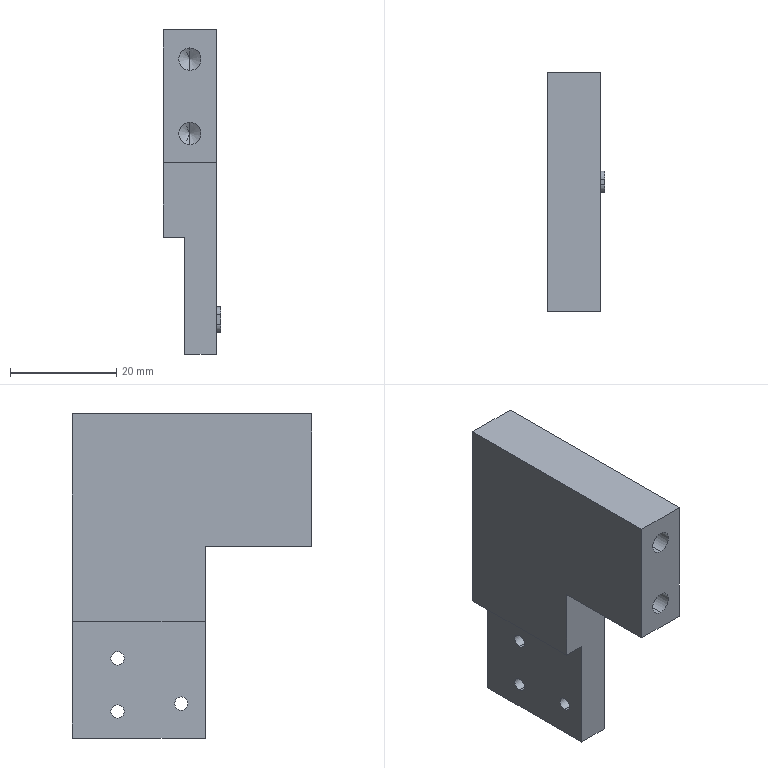Part | SolidWorks | features ICE 4, HoleWzd 3, ExtruThin 1, Fillet 1 | 1 solid | 33 faces | box 10.8 x 45 x 61 mm | volume 17616 mm3 | plane 15 | cylinder 14 | cone 4 | commonest cylinder face diameters 2.5 x6 3 x4 4.2 x4
STEP:
#1=CARTESIAN_POINT('',(10.8,24.5,-30.75));
#2=VERTEX_POINT('',#1);
#3=CARTESIAN_POINT('',(10.8,24.5,-28.25));
#4=VERTEX_POINT('',#3);
#5=CARTESIAN_POINT('',(10.8,24.5,-29.5));
#6=DIRECTION('',(-1.,0.,0.));
#7=DIRECTION('',(0.,0.,1.));
#8=AXIS2_PLACEMENT_3D('',#5,#6,#7);
#9=CIRCLE('',#8,1.25);
#10=EDGE_CURVE('',#2,#4,#9,.T.);
#11=ORIENTED_EDGE('',*,*,#10,.F.);
#12=CARTESIAN_POINT('',(4.,24.5,-30.75));
#13=VERTEX_POINT('',#12);
#14=CARTESIAN_POINT('',(0.,24.5,-30.75));
#15=DIRECTION('',(-1.,0.,0.));
#16=VECTOR('',#15,1000.);
#17=LINE('',#14,#16);
#18=EDGE_CURVE('',#2,#13,#17,.T.);
#19=ORIENTED_EDGE('',*,*,#18,.T.);
#20=CARTESIAN_POINT('',(4.,24.5,-28.25));
#21=VERTEX_POINT('',#20);
#22=CARTESIAN_POINT('',(4.,24.5,-29.5));
#23=DIRECTION('',(1.,0.,0.));
#24=DIRECTION('',(0.,0.,-1.));
#25=AXIS2_PLACEMENT_3D('',#22,#23,#24);
#26=CIRCLE('',#25,1.25);
#27=EDGE_CURVE('',#21,#13,#26,.T.);
#28=ORIENTED_EDGE('',*,*,#27,.F.);
#29=CARTESIAN_POINT('',(0.,24.5,-28.25));
#30=DIRECTION('',(-1.,0.,0.));
#31=VECTOR('',#30,1000.);
#32=LINE('',#29,#31);
#33=EDGE_CURVE('',#4,#21,#32,.T.);
#34=ORIENTED_EDGE('',*,*,#33,.F.);
#35=EDGE_LOOP('',(#11,#19,#28,#34));
#36=FACE_OUTER_BOUND('',#35,.T.);
#37=CARTESIAN_POINT('',(0.,24.5,-29.5));
#38=DIRECTION('',(-1.,0.,0.));
#39=DIRECTION('',(0.,0.,1.));
#40=AXIS2_PLACEMENT_3D('',#37,#38,#39);
#41=CYLINDRICAL_SURFACE('',#40,1.25);
#42=ADVANCED_FACE('',(#36),#41,.F.);
#43=CARTESIAN_POINT('',(4.,36.5,-19.75));
#44=VERTEX_POINT('',#43);
#45=CARTESIAN_POINT('',(4.,36.5,-22.25));
#46=VERTEX_POINT('',#45);
#47=CARTESIAN_POINT('',(4.,36.5,-21.));
#48=DIRECTION('',(1.,0.,0.));
#49=DIRECTION('',(0.,0.,-1.));
#50=AXIS2_PLACEMENT_3D('',#47,#48,#49);
#51=CIRCLE('',#50,1.25);
#52=EDGE_CURVE('',#44,#46,#51,.T.);
#53=ORIENTED_EDGE('',*,*,#52,.F.);
#54=CARTESIAN_POINT('',(10.,36.5,-19.75));
#55=VERTEX_POINT('',#54);
#56=CARTESIAN_POINT('',(10.,36.5,-19.75));
#57=DIRECTION('',(1.,0.,0.));
#58=VECTOR('',#57,1000.);
#59=LINE('',#56,#58);
#60=EDGE_CURVE('',#44,#55,#59,.T.);
#61=ORIENTED_EDGE('',*,*,#60,.T.);
#62=CARTESIAN_POINT('',(10.,36.5,-22.25));
#63=VERTEX_POINT('',#62);
#64=CARTESIAN_POINT('',(10.,36.5,-21.));
#65=DIRECTION('',(1.,0.,0.));
#66=DIRECTION('',(0.,0.,-1.));
#67=AXIS2_PLACEMENT_3D('',#64,#65,#66);
#68=CIRCLE('',#67,1.25);
#69=EDGE_CURVE('',#55,#63,#68,.T.);
#70=ORIENTED_EDGE('',*,*,#69,.T.);
#71=CARTESIAN_POINT('',(10.,36.5,-22.25));
#72=DIRECTION('',(1.,0.,0.));
#73=VECTOR('',#72,1000.);
#74=LINE('',#71,#73);
#75=EDGE_CURVE('',#46,#63,#74,.T.);
#76=ORIENTED_EDGE('',*,*,#75,.F.);
#77=EDGE_LOOP('',(#53,#61,#70,#76));
#78=FACE_OUTER_BOUND('',#77,.T.);
#79=CARTESIAN_POINT('',(10.,36.5,-21.));
#80=DIRECTION('',(1.,0.,0.));
#81=DIRECTION('',(0.,0.,-1.));
#82=AXIS2_PLACEMENT_3D('',#79,#80,#81);
#83=CYLINDRICAL_SURFACE('',#82,1.25);
#84=ADVANCED_FACE('',(#78),#83,.F.);
#85=CARTESIAN_POINT('',(4.,36.5,-29.75));
#86=VERTEX_POINT('',#85);
#87=CARTESIAN_POINT('',(4.,36.5,-32.25));
#88=VERTEX_POINT('',#87);
#89=CARTESIAN_POINT('',(4.,36.5,-31.));
#90=DIRECTION('',(1.,0.,0.));
#91=DIRECTION('',(0.,0.,-1.));
#92=AXIS2_PLACEMENT_3D('',#89,#90,#91);
#93=CIRCLE('',#92,1.25);
#94=EDGE_CURVE('',#86,#88,#93,.T.);
#95=ORIENTED_EDGE('',*,*,#94,.F.);
#96=CARTESIAN_POINT('',(10.,36.5,-29.75));
#97=VERTEX_POINT('',#96);
#98=CARTESIAN_POINT('',(10.,36.5,-29.75));
#99=DIRECTION('',(1.,0.,0.));
#100=VECTOR('',#99,1000.);
#101=LINE('',#98,#100);
#102=EDGE_CURVE('',#86,#97,#101,.T.);
#103=ORIENTED_EDGE('',*,*,#102,.T.);
#104=CARTESIAN_POINT('',(10.,36.5,-32.25));
#105=VERTEX_POINT('',#104);
#106=CARTESIAN_POINT('',(10.,36.5,-31.));
#107=DIRECTION('',(1.,0.,0.));
#108=DIRECTION('',(0.,0.,-1.));
#109=AXIS2_PLACEMENT_3D('',#106,#107,#108);
#110=CIRCLE('',#109,1.25);
#111=EDGE_CURVE('',#97,#105,#110,.T.);
#112=ORIENTED_EDGE('',*,*,#111,.T.);
#113=CARTESIAN_POINT('',(10.,36.5,-32.25));
#114=DIRECTION('',(1.,0.,0.));
#115=VECTOR('',#114,1000.);
#116=LINE('',#113,#115);
#117=EDGE_CURVE('',#88,#105,#116,.T.);
#118=ORIENTED_EDGE('',*,*,#117,.F.);
#119=EDGE_LOOP('',(#95,#103,#112,#118));
#120=FACE_OUTER_BOUND('',#119,.T.);
#121=CARTESIAN_POINT('',(10.,36.5,-31.));
#122=DIRECTION('',(1.,0.,0.));
#123=DIRECTION('',(0.,0.,-1.));
#124=AXIS2_PLACEMENT_3D('',#121,#122,#123);
#125=CYLINDRICAL_SURFACE('',#124,1.25);
#126=ADVANCED_FACE('',(#120),#125,.F.);
#127=CARTESIAN_POINT('',(5.,12.4,7.6));
#128=VERTEX_POINT('',#127);
#129=CARTESIAN_POINT('',(5.,12.4,3.4));
#130=VERTEX_POINT('',#129);
#131=CARTESIAN_POINT('',(5.,12.4,5.5));
#132=DIRECTION('',(0.,-1.,0.));
#133=DIRECTION('',(0.,0.,-1.));
#134=AXIS2_PLACEMENT_3D('',#131,#132,#133);
#135=CIRCLE('',#134,2.1);
#136=EDGE_CURVE('',#128,#130,#135,.T.);
#137=ORIENTED_EDGE('',*,*,#136,.F.);
#138=CARTESIAN_POINT('',(5.,0.,7.6));
#139=VERTEX_POINT('',#138);
#140=CARTESIAN_POINT('',(5.,0.,7.6));
#141=DIRECTION('',(0.,-1.,0.));
#142=VECTOR('',#141,1000.);
#143=LINE('',#140,#142);
#144=EDGE_CURVE('',#128,#139,#143,.T.);
#145=ORIENTED_EDGE('',*,*,#144,.T.);
#146=CARTESIAN_POINT('',(5.,0.,3.4));
#147=VERTEX_POINT('',#146);
#148=CARTESIAN_POINT('',(5.,0.,5.5));
#149=DIRECTION('',(0.,-1.,0.));
#150=DIRECTION('',(0.,0.,-1.));
#151=AXIS2_PLACEMENT_3D('',#148,#149,#150);
#152=CIRCLE('',#151,2.1);
#153=EDGE_CURVE('',#139,#147,#152,.T.);
#154=ORIENTED_EDGE('',*,*,#153,.T.);
#155=CARTESIAN_POINT('',(5.,0.,3.4));
#156=DIRECTION('',(0.,-1.,0.));
#157=VECTOR('',#156,1000.);
#158=LINE('',#155,#157);
#159=EDGE_CURVE('',#130,#147,#158,.T.);
#160=ORIENTED_EDGE('',*,*,#159,.F.);
#161=EDGE_LOOP('',(#137,#145,#154,#160));
#162=FACE_OUTER_BOUND('',#161,.T.);
#163=CARTESIAN_POINT('',(5.,0.,5.5));
#164=DIRECTION('',(0.,-1.,0.));
#165=DIRECTION('',(0.,0.,-1.));
#166=AXIS2_PLACEMENT_3D('',#163,#164,#165);
#167=CYLINDRICAL_SURFACE('',#166,2.1);
#168=ADVANCED_FACE('',(#162),#167,.F.);
#169=CARTESIAN_POINT('',(5.,13.662,5.5));
#170=VERTEX_POINT('',#169);
#171=CARTESIAN_POINT('',(5.,12.4,3.4));
#172=DIRECTION('',(0.,-0.515,-0.8572));
#173=VECTOR('',#172,1000.);
#174=LINE('',#171,#173);
#175=EDGE_CURVE('',#170,#130,#174,.T.);
#176=ORIENTED_EDGE('',*,*,#175,.F.);
#177=CARTESIAN_POINT('',(5.,12.4,7.6));
#178=DIRECTION('',(0.,-0.515,0.8572));
#179=VECTOR('',#178,1000.);
#180=LINE('',#177,#179);
#181=EDGE_CURVE('',#170,#128,#180,.T.);
#182=ORIENTED_EDGE('',*,*,#181,.T.);
#183=ORIENTED_EDGE('',*,*,#136,.T.);
#184=EDGE_LOOP('',(#176,#182,#183));
#185=FACE_OUTER_BOUND('',#184,.T.);
#186=CARTESIAN_POINT('',(5.,12.4,5.5));
#187=DIRECTION('',(0.,-1.,0.));
#188=DIRECTION('',(0.,0.,-1.));
#189=AXIS2_PLACEMENT_3D('',#186,#187,#188);
#190=CONICAL_SURFACE('',#189,2.1,1.03);
#191=ADVANCED_FACE('',(#185),#190,.F.);
#192=CARTESIAN_POINT('',(5.,12.4,21.6));
#193=VERTEX_POINT('',#192);
#194=CARTESIAN_POINT('',(5.,12.4,17.4));
#195=VERTEX_POINT('',#194);
#196=CARTESIAN_POINT('',(5.,12.4,19.5));
#197=DIRECTION('',(0.,-1.,0.));
#198=DIRECTION('',(0.,0.,-1.));
#199=AXIS2_PLACEMENT_3D('',#196,#197,#198);
#200=CIRCLE('',#199,2.1);
#201=EDGE_CURVE('',#193,#195,#200,.T.);
#202=ORIENTED_EDGE('',*,*,#201,.F.);
#203=CARTESIAN_POINT('',(5.,0.,21.6));
#204=VERTEX_POINT('',#203);
#205=CARTESIAN_POINT('',(5.,0.,21.6));
#206=DIRECTION('',(0.,-1.,0.));
#207=VECTOR('',#206,1000.);
#208=LINE('',#205,#207);
#209=EDGE_CURVE('',#193,#204,#208,.T.);
#210=ORIENTED_EDGE('',*,*,#209,.T.);
#211=CARTESIAN_POINT('',(5.,0.,17.4));
#212=VERTEX_POINT('',#211);
#213=CARTESIAN_POINT('',(5.,0.,19.5));
#214=DIRECTION('',(0.,-1.,0.));
#215=DIRECTION('',(0.,0.,-1.));
#216=AXIS2_PLACEMENT_3D('',#213,#214,#215);
#217=CIRCLE('',#216,2.1);
#218=EDGE_CURVE('',#204,#212,#217,.T.);
#219=ORIENTED_EDGE('',*,*,#218,.T.);
#220=CARTESIAN_POINT('',(5.,0.,17.4));
#221=DIRECTION('',(0.,-1.,0.));
#222=VECTOR('',#221,1000.);
#223=LINE('',#220,#222);
#224=EDGE_CURVE('',#195,#212,#223,.T.);
#225=ORIENTED_EDGE('',*,*,#224,.F.);
#226=EDGE_LOOP('',(#202,#210,#219,#225));
#227=FACE_OUTER_BOUND('',#226,.T.);
#228=CARTESIAN_POINT('',(5.,0.,19.5));
#229=DIRECTION('',(0.,-1.,0.));
#230=DIRECTION('',(0.,0.,-1.));
#231=AXIS2_PLACEMENT_3D('',#228,#229,#230);
#232=CYLINDRICAL_SURFACE('',#231,2.1);
#233=ADVANCED_FACE('',(#227),#232,.F.);
#234=CARTESIAN_POINT('',(5.,13.662,19.5));
#235=VERTEX_POINT('',#234);
#236=CARTESIAN_POINT('',(5.,12.4,17.4));
#237=DIRECTION('',(0.,-0.515,-0.8572));
#238=VECTOR('',#237,1000.);
#239=LINE('',#236,#238);
#240=EDGE_CURVE('',#235,#195,#239,.T.);
#241=ORIENTED_EDGE('',*,*,#240,.F.);
#242=CARTESIAN_POINT('',(5.,12.4,21.6));
#243=DIRECTION('',(0.,-0.515,0.8572));
#244=VECTOR('',#243,1000.);
#245=LINE('',#242,#244);
#246=EDGE_CURVE('',#235,#193,#245,.T.);
#247=ORIENTED_EDGE('',*,*,#246,.T.);
#248=ORIENTED_EDGE('',*,*,#201,.T.);
#249=EDGE_LOOP('',(#241,#247,#248));
#250=FACE_OUTER_BOUND('',#249,.T.);
#251=CARTESIAN_POINT('',(5.,12.4,19.5));
#252=DIRECTION('',(0.,-1.,0.));
#253=DIRECTION('',(0.,0.,-1.));
#254=AXIS2_PLACEMENT_3D('',#251,#252,#253);
#255=CONICAL_SURFACE('',#254,2.1,1.03);
#256=ADVANCED_FACE('',(#250),#255,.F.);
#257=CARTESIAN_POINT('',(10.,0.,0.));
#258=VERTEX_POINT('',#257);
#259=CARTESIAN_POINT('',(10.,0.,25.));
#260=VERTEX_POINT('',#259);
#261=CARTESIAN_POINT('',(10.,0.,25.));
#262=DIRECTION('',(0.,0.,1.));
#263=VECTOR('',#262,1000.);
#264=LINE('',#261,#263);
#265=EDGE_CURVE('',#258,#260,#264,.T.);
#266=ORIENTED_EDGE('',*,*,#265,.F.);
#267=CARTESIAN_POINT('',(10.,20.,0.));
#268=VERTEX_POINT('',#267);
#269=CARTESIAN_POINT('',(10.,0.,0.));
#270=DIRECTION('',(0.,1.,0.));
#271=VECTOR('',#270,1000.);
#272=LINE('',#269,#271);
#273=EDGE_CURVE('',#258,#268,#272,.T.);
#274=ORIENTED_EDGE('',*,*,#273,.T.);
#275=CARTESIAN_POINT('',(10.,20.,-36.));
#276=VERTEX_POINT('',#275);
#277=CARTESIAN_POINT('',(10.,20.,0.));
#278=DIRECTION('',(0.,0.,-1.));
#279=VECTOR('',#278,1000.);
#280=LINE('',#277,#279);
#281=EDGE_CURVE('',#268,#276,#280,.T.);
#282=ORIENTED_EDGE('',*,*,#281,.T.);
#283=CARTESIAN_POINT('',(10.,45.,-36.));
#284=VERTEX_POINT('',#283);
#285=CARTESIAN_POINT('',(10.,45.,-36.));
#286=DIRECTION('',(0.,1.,0.));
#287=VECTOR('',#286,1000.);
#288=LINE('',#285,#287);
#289=EDGE_CURVE('',#276,#284,#288,.T.);
#290=ORIENTED_EDGE('',*,*,#289,.T.);
#291=CARTESIAN_POINT('',(10.,45.,25.));
#292=VERTEX_POINT('',#291);
#293=CARTESIAN_POINT('',(10.,45.,25.));
#294=DIRECTION('',(0.,0.,-1.));
#295=VECTOR('',#294,1000.);
#296=LINE('',#293,#295);
#297=EDGE_CURVE('',#292,#284,#296,.T.);
#298=ORIENTED_EDGE('',*,*,#297,.F.);
#299=CARTESIAN_POINT('',(10.,0.,25.));
#300=DIRECTION('',(0.,1.,0.));
#301=VECTOR('',#300,1000.);
#302=LINE('',#299,#301);
#303=EDGE_CURVE('',#260,#292,#302,.T.);
#304=ORIENTED_EDGE('',*,*,#303,.F.);
#305=EDGE_LOOP('',(#266,#274,#282,#290,#298,#304));
#306=FACE_OUTER_BOUND('',#305,.T.);
#307=CARTESIAN_POINT('',(10.,36.5,-31.));
#308=DIRECTION('',(1.,0.,0.));
#309=DIRECTION('',(0.,0.,-1.));
#310=AXIS2_PLACEMENT_3D('',#307,#308,#309);
#311=CIRCLE('',#310,1.25);
#312=EDGE_CURVE('',#105,#97,#311,.T.);
#313=ORIENTED_EDGE('',*,*,#312,.F.);
#314=ORIENTED_EDGE('',*,*,#111,.F.);
#315=EDGE_LOOP('',(#313,#314));
#316=FACE_BOUND('',#315,.T.);
#317=CARTESIAN_POINT('',(10.,36.5,-21.));
#318=DIRECTION('',(1.,0.,0.));
#319=DIRECTION('',(0.,0.,-1.));
#320=AXIS2_PLACEMENT_3D('',#317,#318,#319);
#321=CIRCLE('',#320,1.25);
#322=EDGE_CURVE('',#63,#55,#321,.T.);
#323=ORIENTED_EDGE('',*,*,#322,.F.);
#324=ORIENTED_EDGE('',*,*,#69,.F.);
#325=EDGE_LOOP('',(#323,#324));
#326=FACE_BOUND('',#325,.T.);
#327=CARTESIAN_POINT('',(10.,24.,-31.9));
#328=VERTEX_POINT('',#327);
#329=CARTESIAN_POINT('',(10.,25.,-31.9));
#330=VERTEX_POINT('',#329);
#331=CARTESIAN_POINT('',(10.,26.5,-31.9));
#332=DIRECTION('',(0.,1.,0.));
#333=VECTOR('',#332,1000.);
#334=LINE('',#331,#333);
#335=EDGE_CURVE('',#328,#330,#334,.T.);
#336=ORIENTED_EDGE('',*,*,#335,.F.);
#337=CARTESIAN_POINT('',(10.,22.5,-30.4));
#338=VERTEX_POINT('',#337);
#339=CARTESIAN_POINT('',(10.,24.,-30.4));
#340=DIRECTION('',(-1.,0.,0.));
#341=DIRECTION('',(0.,0.,1.));
#342=AXIS2_PLACEMENT_3D('',#339,#340,#341);
#343=CIRCLE('',#342,1.5);
#344=EDGE_CURVE('',#328,#338,#343,.T.);
#345=ORIENTED_EDGE('',*,*,#344,.T.);
#346=CARTESIAN_POINT('',(10.,22.5,-28.6));
#347=VERTEX_POINT('',#346);
#348=CARTESIAN_POINT('',(10.,22.5,-27.1));
#349=DIRECTION('',(0.,0.,-1.));
#350=VECTOR('',#349,1000.);
#351=LINE('',#348,#350);
#352=EDGE_CURVE('',#347,#338,#351,.T.);
#353=ORIENTED_EDGE('',*,*,#352,.F.);
#354=CARTESIAN_POINT('',(10.,24.,-27.1));
#355=VERTEX_POINT('',#354);
#356=CARTESIAN_POINT('',(10.,24.,-28.6));
#357=DIRECTION('',(-1.,0.,0.));
#358=DIRECTION('',(0.,0.,1.));
#359=AXIS2_PLACEMENT_3D('',#356,#357,#358);
#360=CIRCLE('',#359,1.5);
#361=EDGE_CURVE('',#347,#355,#360,.T.);
#362=ORIENTED_EDGE('',*,*,#361,.T.);
#363=CARTESIAN_POINT('',(10.,25.,-27.1));
#364=VERTEX_POINT('',#363);
#365=CARTESIAN_POINT('',(10.,26.5,-27.1));
#366=DIRECTION('',(0.,-1.,0.));
#367=VECTOR('',#366,1000.);
#368=LINE('',#365,#367);
#369=EDGE_CURVE('',#364,#355,#368,.T.);
#370=ORIENTED_EDGE('',*,*,#369,.F.);
#371=CARTESIAN_POINT('',(10.,26.5,-28.6));
#372=VERTEX_POINT('',#371);
#373=CARTESIAN_POINT('',(10.,25.,-28.6));
#374=DIRECTION('',(-1.,0.,0.));
#375=DIRECTION('',(0.,0.,1.));
#376=AXIS2_PLACEMENT_3D('',#373,#374,#375);
#377=CIRCLE('',#376,1.5);
#378=EDGE_CURVE('',#364,#372,#377,.T.);
#379=ORIENTED_EDGE('',*,*,#378,.T.);
#380=CARTESIAN_POINT('',(10.,26.5,-30.4));
#381=VERTEX_POINT('',#380);
#382=CARTESIAN_POINT('',(10.,26.5,-27.1));
#383=DIRECTION('',(0.,0.,1.));
#384=VECTOR('',#383,1000.);
#385=LINE('',#382,#384);
#386=EDGE_CURVE('',#381,#372,#385,.T.);
#387=ORIENTED_EDGE('',*,*,#386,.F.);
#388=CARTESIAN_POINT('',(10.,25.,-30.4));
#389=DIRECTION('',(-1.,0.,0.));
#390=DIRECTION('',(0.,0.,1.));
#391=AXIS2_PLACEMENT_3D('',#388,#389,#390);
#392=CIRCLE('',#391,1.5);
#393=EDGE_CURVE('',#381,#330,#392,.T.);
#394=ORIENTED_EDGE('',*,*,#393,.T.);
#395=EDGE_LOOP('',(#336,#345,#353,#362,#370,#379,#387,#394));
#396=FACE_BOUND('',#395,.T.);
#397=CARTESIAN_POINT('',(10.,0.,25.));
#398=DIRECTION('',(-1.,0.,0.));
#399=DIRECTION('',(0.,0.,1.));
#400=AXIS2_PLACEMENT_3D('',#397,#398,#399);
#401=PLANE('',#400);
#402=ADVANCED_FACE('',(#306,#316,#326,#396),#401,.F.);
#403=CARTESIAN_POINT('',(0.,0.,25.));
#404=VERTEX_POINT('',#403);
#405=CARTESIAN_POINT('',(0.,0.,25.));
#406=DIRECTION('',(-1.,0.,0.));
#407=VECTOR('',#406,1000.);
#408=LINE('',#405,#407);
#409=EDGE_CURVE('',#260,#404,#408,.T.);
#410=ORIENTED_EDGE('',*,*,#409,.F.);
#411=ORIENTED_EDGE('',*,*,#303,.T.);
#412=CARTESIAN_POINT('',(0.,45.,25.));
#413=VERTEX_POINT('',#412);
#414=CARTESIAN_POINT('',(0.,45.,25.));
#415=DIRECTION('',(1.,0.,0.));
#416=VECTOR('',#415,1000.);
#417=LINE('',#414,#416);
#418=EDGE_CURVE('',#413,#292,#417,.T.);
#419=ORIENTED_EDGE('',*,*,#418,.F.);
#420=CARTESIAN_POINT('',(0.,0.,25.));
#421=DIRECTION('',(0.,1.,0.));
#422=VECTOR('',#421,1000.);
#423=LINE('',#420,#422);
#424=EDGE_CURVE('',#404,#413,#423,.T.);
#425=ORIENTED_EDGE('',*,*,#424,.F.);
#426=EDGE_LOOP('',(#410,#411,#419,#425));
#427=FACE_OUTER_BOUND('',#426,.T.);
#428=CARTESIAN_POINT('',(0.,0.,25.));
#429=DIRECTION('',(0.,0.,-1.));
#430=DIRECTION('',(-1.,0.,0.));
#431=AXIS2_PLACEMENT_3D('',#428,#429,#430);
#432=PLANE('',#431);
#433=ADVANCED_FACE('',(#427),#432,.F.);
#434=ORIENTED_EDGE('',*,*,#273,.F.);
#435=CARTESIAN_POINT('',(0.,0.,0.));
#436=VERTEX_POINT('',#435);
#437=CARTESIAN_POINT('',(0.,0.,0.));
#438=DIRECTION('',(-1.,0.,0.));
#439=VECTOR('',#438,1000.);
#440=LINE('',#437,#439);
#441=EDGE_CURVE('',#258,#436,#440,.T.);
#442=ORIENTED_EDGE('',*,*,#441,.T.);
#443=CARTESIAN_POINT('',(0.,20.,0.));
#444=VERTEX_POINT('',#443);
#445=CARTESIAN_POINT('',(0.,0.,0.));
#446=DIRECTION('',(0.,1.,0.));
#447=VECTOR('',#446,1000.);
#448=LINE('',#445,#447);
#449=EDGE_CURVE('',#436,#444,#448,.T.);
#450=ORIENTED_EDGE('',*,*,#449,.T.);
#451=CARTESIAN_POINT('',(53.829,20.,0.));
#452=DIRECTION('',(-1.,0.,0.));
#453=VECTOR('',#452,1000.);
#454=LINE('',#451,#453);
#455=EDGE_CURVE('',#268,#444,#454,.T.);
#456=ORIENTED_EDGE('',*,*,#455,.F.);
#457=EDGE_LOOP('',(#434,#442,#450,#456));
#458=FACE_OUTER_BOUND('',#457,.T.);
#459=CARTESIAN_POINT('',(0.,0.,0.));
#460=DIRECTION('',(0.,0.,-1.));
#461=DIRECTION('',(-1.,0.,0.));
#462=AXIS2_PLACEMENT_3D('',#459,#460,#461);
#463=PLANE('',#462);
#464=ADVANCED_FACE('',(#458),#463,.T.);
#465=CARTESIAN_POINT('',(4.,45.,-14.));
#466=VERTEX_POINT('',#465);
#467=CARTESIAN_POINT('',(4.,45.,-36.));
#468=VERTEX_POINT('',#467);
#469=CARTESIAN_POINT('',(4.,45.,-36.));
#470=DIRECTION('',(0.,0.,-1.));
#471=VECTOR('',#470,1000.);
#472=LINE('',#469,#471);
#473=EDGE_CURVE('',#466,#468,#472,.T.);
#474=ORIENTED_EDGE('',*,*,#473,.F.);
#475=CARTESIAN_POINT('',(0.,45.,-14.));
#476=VERTEX_POINT('',#475);
#477=CARTESIAN_POINT('',(0.,45.,-14.));
#478=DIRECTION('',(1.,0.,0.));
#479=VECTOR('',#478,1000.);
#480=LINE('',#477,#479);
#481=EDGE_CURVE('',#476,#466,#480,.T.);
#482=ORIENTED_EDGE('',*,*,#481,.F.);
#483=CARTESIAN_POINT('',(0.,45.,25.));
#484=DIRECTION('',(0.,0.,-1.));
#485=VECTOR('',#484,1000.);
#486=LINE('',#483,#485);
#487=EDGE_CURVE('',#413,#476,#486,.T.);
#488=ORIENTED_EDGE('',*,*,#487,.F.);
#489=ORIENTED_EDGE('',*,*,#418,.T.);
#490=ORIENTED_EDGE('',*,*,#297,.T.);
#491=CARTESIAN_POINT('',(53.829,45.,-36.));
#492=DIRECTION('',(-1.,0.,0.));
#493=VECTOR('',#492,1000.);
#494=LINE('',#491,#493);
#495=EDGE_CURVE('',#284,#468,#494,.T.);
#496=ORIENTED_EDGE('',*,*,#495,.T.);
#497=EDGE_LOOP('',(#474,#482,#488,#489,#490,#496));
#498=FACE_OUTER_BOUND('',#497,.T.);
#499=CARTESIAN_POINT('',(0.,45.,25.));
#500=DIRECTION('',(0.,1.,0.));
#501=DIRECTION('',(0.,0.,1.));
#502=AXIS2_PLACEMENT_3D('',#499,#500,#501);
#503=PLANE('',#502);
#504=ADVANCED_FACE('',(#498),#503,.T.);
#505=CARTESIAN_POINT('',(0.,20.,-14.));
#506=VERTEX_POINT('',#505);
#507=CARTESIAN_POINT('',(0.,-10.,-14.));
#508=DIRECTION('',(0.,1.,0.));
#509=VECTOR('',#508,1000.);
#510=LINE('',#507,#509);
#511=EDGE_CURVE('',#506,#476,#510,.T.);
#512=ORIENTED_EDGE('',*,*,#511,.F.);
#513=CARTESIAN_POINT('',(0.,20.,0.));
#514=DIRECTION('',(0.,0.,1.));
#515=VECTOR('',#514,1000.);
#516=LINE('',#513,#515);
#517=EDGE_CURVE('',#506,#444,#516,.T.);
#518=ORIENTED_EDGE('',*,*,#517,.T.);
#519=ORIENTED_EDGE('',*,*,#449,.F.);
#520=CARTESIAN_POINT('',(0.,0.,25.));
#521=DIRECTION('',(0.,0.,-1.));
#522=VECTOR('',#521,1000.);
#523=LINE('',#520,#522);
#524=EDGE_CURVE('',#404,#436,#523,.T.);
#525=ORIENTED_EDGE('',*,*,#524,.F.);
#526=ORIENTED_EDGE('',*,*,#424,.T.);
#527=ORIENTED_EDGE('',*,*,#487,.T.);
#528=EDGE_LOOP('',(#512,#518,#519,#525,#526,#527));
#529=FACE_OUTER_BOUND('',#528,.T.);
#530=CARTESIAN_POINT('',(0.,0.,25.));
#531=DIRECTION('',(-1.,0.,0.));
#532=DIRECTION('',(0.,0.,1.));
#533=AXIS2_PLACEMENT_3D('',#530,#531,#532);
#534=PLANE('',#533);
#535=ADVANCED_FACE('',(#529),#534,.T.);
#536=CARTESIAN_POINT('',(4.,20.,-36.));
#537=VERTEX_POINT('',#536);
#538=CARTESIAN_POINT('',(4.,20.,-14.));
#539=VERTEX_POINT('',#538);
#540=CARTESIAN_POINT('',(4.,20.,0.));
#541=DIRECTION('',(0.,0.,1.));
#542=VECTOR('',#541,1000.);
#543=LINE('',#540,#542);
#544=EDGE_CURVE('',#537,#539,#543,.T.);
#545=ORIENTED_EDGE('',*,*,#544,.F.);
#546=CARTESIAN_POINT('',(53.829,20.,-36.));
#547=DIRECTION('',(-1.,0.,0.));
#548=VECTOR('',#547,1000.);
#549=LINE('',#546,#548);
#550=EDGE_CURVE('',#276,#537,#549,.T.);
#551=ORIENTED_EDGE('',*,*,#550,.F.);
#552=ORIENTED_EDGE('',*,*,#281,.F.);
#553=ORIENTED_EDGE('',*,*,#455,.T.);
#554=ORIENTED_EDGE('',*,*,#517,.F.);
#555=CARTESIAN_POINT('',(53.829,20.,-14.));
#556=DIRECTION('',(-1.,0.,0.));
#557=VECTOR('',#556,1000.);
#558=LINE('',#555,#557);
#559=EDGE_CURVE('',#539,#506,#558,.T.);
#560=ORIENTED_EDGE('',*,*,#559,.F.);
#561=EDGE_LOOP('',(#545,#551,#552,#553,#554,#560));
#562=FACE_OUTER_BOUND('',#561,.T.);
#563=CARTESIAN_POINT('',(53.829,20.,0.));
#564=DIRECTION('',(0.,-1.,0.));
#565=DIRECTION('',(0.,0.,-1.));
#566=AXIS2_PLACEMENT_3D('',#563,#564,#565);
#567=PLANE('',#566);
#568=ADVANCED_FACE('',(#562),#567,.T.);
#569=CARTESIAN_POINT('',(4.,45.,-36.));
#570=DIRECTION('',(0.,-1.,0.));
#571=VECTOR('',#570,1000.);
#572=LINE('',#569,#571);
#573=EDGE_CURVE('',#468,#537,#572,.T.);
#574=ORIENTED_EDGE('',*,*,#573,.F.);
#575=ORIENTED_EDGE('',*,*,#495,.F.);
#576=ORIENTED_EDGE('',*,*,#289,.F.);
#577=ORIENTED_EDGE('',*,*,#550,.T.);
#578=EDGE_LOOP('',(#574,#575,#576,#577));
#579=FACE_OUTER_BOUND('',#578,.T.);
#580=CARTESIAN_POINT('',(53.829,45.,-36.));
#581=DIRECTION('',(0.,0.,-1.));
#582=DIRECTION('',(0.,1.,0.));
#583=AXIS2_PLACEMENT_3D('',#580,#581,#582);
#584=PLANE('',#583);
#585=ADVANCED_FACE('',(#579),#584,.T.);
#586=ORIENTED_EDGE('',*,*,#27,.T.);
#587=CARTESIAN_POINT('',(4.,24.5,-29.5));
#588=DIRECTION('',(1.,0.,0.));
#589=DIRECTION('',(0.,0.,-1.));
#590=AXIS2_PLACEMENT_3D('',#587,#588,#589);
#591=CIRCLE('',#590,1.25);
#592=EDGE_CURVE('',#13,#21,#591,.T.);
#593=ORIENTED_EDGE('',*,*,#592,.T.);
#594=EDGE_LOOP('',(#586,#593));
#595=FACE_BOUND('',#594,.T.);
#596=CARTESIAN_POINT('',(4.,36.5,-21.));
#597=DIRECTION('',(1.,0.,0.));
#598=DIRECTION('',(0.,0.,-1.));
#599=AXIS2_PLACEMENT_3D('',#596,#597,#598);
#600=CIRCLE('',#599,1.25);
#601=EDGE_CURVE('',#46,#44,#600,.T.);
#602=ORIENTED_EDGE('',*,*,#601,.T.);
#603=ORIENTED_EDGE('',*,*,#52,.T.);
#604=EDGE_LOOP('',(#602,#603));
#605=FACE_BOUND('',#604,.T.);
#606=CARTESIAN_POINT('',(4.,36.5,-31.));
#607=DIRECTION('',(1.,0.,0.));
#608=DIRECTION('',(0.,0.,-1.));
#609=AXIS2_PLACEMENT_3D('',#606,#607,#608);
#610=CIRCLE('',#609,1.25);
#611=EDGE_CURVE('',#88,#86,#610,.T.);
#612=ORIENTED_EDGE('',*,*,#611,.T.);
#613=ORIENTED_EDGE('',*,*,#94,.T.);
#614=EDGE_LOOP('',(#612,#613));
#615=FACE_BOUND('',#614,.T.);
#616=ORIENTED_EDGE('',*,*,#544,.T.);
#617=CARTESIAN_POINT('',(4.,-10.,-14.));
#618=DIRECTION('',(0.,1.,0.));
#619=VECTOR('',#618,1000.);
#620=LINE('',#617,#619);
#621=EDGE_CURVE('',#539,#466,#620,.T.);
#622=ORIENTED_EDGE('',*,*,#621,.T.);
#623=ORIENTED_EDGE('',*,*,#473,.T.);
#624=ORIENTED_EDGE('',*,*,#573,.T.);
#625=EDGE_LOOP('',(#616,#622,#623,#624));
#626=FACE_OUTER_BOUND('',#625,.T.);
#627=CARTESIAN_POINT('',(4.,-10.,-36.));
#628=DIRECTION('',(1.,0.,0.));
#629=DIRECTION('',(0.,0.,-1.));
#630=AXIS2_PLACEMENT_3D('',#627,#628,#629);
#631=PLANE('',#630);
#632=ADVANCED_FACE('',(#595,#605,#615,#626),#631,.F.);
#633=ORIENTED_EDGE('',*,*,#559,.T.);
#634=ORIENTED_EDGE('',*,*,#511,.T.);
#635=ORIENTED_EDGE('',*,*,#481,.T.);
#636=ORIENTED_EDGE('',*,*,#621,.F.);
#637=EDGE_LOOP('',(#633,#634,#635,#636));
#638=FACE_OUTER_BOUND('',#637,.T.);
#639=CARTESIAN_POINT('',(0.,-10.,-14.));
#640=DIRECTION('',(0.,0.,1.));
#641=DIRECTION('',(1.,0.,0.));
#642=AXIS2_PLACEMENT_3D('',#639,#640,#641);
#643=PLANE('',#642);
#644=ADVANCED_FACE('',(#638),#643,.F.);
#645=CARTESIAN_POINT('',(5.,0.,5.5));
#646=DIRECTION('',(0.,-1.,0.));
#647=DIRECTION('',(0.,0.,-1.));
#648=AXIS2_PLACEMENT_3D('',#645,#646,#647);
#649=CIRCLE('',#648,2.1);
#650=EDGE_CURVE('',#147,#139,#649,.T.);
#651=ORIENTED_EDGE('',*,*,#650,.F.);
#652=ORIENTED_EDGE('',*,*,#153,.F.);
#653=EDGE_LOOP('',(#651,#652));
#654=FACE_BOUND('',#653,.T.);
#655=CARTESIAN_POINT('',(5.,0.,19.5));
#656=DIRECTION('',(0.,-1.,0.));
#657=DIRECTION('',(0.,0.,-1.));
#658=AXIS2_PLACEMENT_3D('',#655,#656,#657);
#659=CIRCLE('',#658,2.1);
#660=EDGE_CURVE('',#212,#204,#659,.T.);
#661=ORIENTED_EDGE('',*,*,#660,.F.);
#662=ORIENTED_EDGE('',*,*,#218,.F.);
#663=EDGE_LOOP('',(#661,#662));
#664=FACE_BOUND('',#663,.T.);
#665=ORIENTED_EDGE('',*,*,#441,.F.);
#666=ORIENTED_EDGE('',*,*,#265,.T.);
#667=ORIENTED_EDGE('',*,*,#409,.T.);
#668=ORIENTED_EDGE('',*,*,#524,.T.);
#669=EDGE_LOOP('',(#665,#666,#667,#668));
#670=FACE_OUTER_BOUND('',#669,.T.);
#671=CARTESIAN_POINT('',(0.,0.,0.));
#672=DIRECTION('',(0.,-1.,0.));
#673=DIRECTION('',(0.,0.,-1.));
#674=AXIS2_PLACEMENT_3D('',#671,#672,#673);
#675=PLANE('',#674);
#676=ADVANCED_FACE('',(#654,#664,#670),#675,.T.);
#677=ORIENTED_EDGE('',*,*,#246,.F.);
#678=ORIENTED_EDGE('',*,*,#240,.T.);
#679=CARTESIAN_POINT('',(5.,12.4,19.5));
#680=DIRECTION('',(0.,-1.,0.));
#681=DIRECTION('',(0.,0.,-1.));
#682=AXIS2_PLACEMENT_3D('',#679,#680,#681);
#683=CIRCLE('',#682,2.1);
#684=EDGE_CURVE('',#195,#193,#683,.T.);
#685=ORIENTED_EDGE('',*,*,#684,.T.);
#686=EDGE_LOOP('',(#677,#678,#685));
#687=FACE_OUTER_BOUND('',#686,.T.);
#688=CARTESIAN_POINT('',(5.,12.4,19.5));
#689=DIRECTION('',(0.,-1.,0.));
#690=DIRECTION('',(0.,0.,-1.));
#691=AXIS2_PLACEMENT_3D('',#688,#689,#690);
#692=CONICAL_SURFACE('',#691,2.1,1.03);
#693=ADVANCED_FACE('',(#687),#692,.F.);
#694=ORIENTED_EDGE('',*,*,#209,.F.);
#695=ORIENTED_EDGE('',*,*,#684,.F.);
#696=ORIENTED_EDGE('',*,*,#224,.T.);
#697=ORIENTED_EDGE('',*,*,#660,.T.);
#698=EDGE_LOOP('',(#694,#695,#696,#697));
#699=FACE_OUTER_BOUND('',#698,.T.);
#700=CARTESIAN_POINT('',(5.,0.,19.5));
#701=DIRECTION('',(0.,-1.,0.));
#702=DIRECTION('',(0.,0.,-1.));
#703=AXIS2_PLACEMENT_3D('',#700,#701,#702);
#704=CYLINDRICAL_SURFACE('',#703,2.1);
#705=ADVANCED_FACE('',(#699),#704,.F.);
#706=ORIENTED_EDGE('',*,*,#181,.F.);
#707=ORIENTED_EDGE('',*,*,#175,.T.);
#708=CARTESIAN_POINT('',(5.,12.4,5.5));
#709=DIRECTION('',(0.,-1.,0.));
#710=DIRECTION('',(0.,0.,-1.));
#711=AXIS2_PLACEMENT_3D('',#708,#709,#710);
#712=CIRCLE('',#711,2.1);
#713=EDGE_CURVE('',#130,#128,#712,.T.);
#714=ORIENTED_EDGE('',*,*,#713,.T.);
#715=EDGE_LOOP('',(#706,#707,#714));
#716=FACE_OUTER_BOUND('',#715,.T.);
#717=CARTESIAN_POINT('',(5.,12.4,5.5));
#718=DIRECTION('',(0.,-1.,0.));
#719=DIRECTION('',(0.,0.,-1.));
#720=AXIS2_PLACEMENT_3D('',#717,#718,#719);
#721=CONICAL_SURFACE('',#720,2.1,1.03);
#722=ADVANCED_FACE('',(#716),#721,.F.);
#723=ORIENTED_EDGE('',*,*,#144,.F.);
#724=ORIENTED_EDGE('',*,*,#713,.F.);
#725=ORIENTED_EDGE('',*,*,#159,.T.);
#726=ORIENTED_EDGE('',*,*,#650,.T.);
#727=EDGE_LOOP('',(#723,#724,#725,#726));
#728=FACE_OUTER_BOUND('',#727,.T.);
#729=CARTESIAN_POINT('',(5.,0.,5.5));
#730=DIRECTION('',(0.,-1.,0.));
#731=DIRECTION('',(0.,0.,-1.));
#732=AXIS2_PLACEMENT_3D('',#729,#730,#731);
#733=CYLINDRICAL_SURFACE('',#732,2.1);
#734=ADVANCED_FACE('',(#728),#733,.F.);
#735=ORIENTED_EDGE('',*,*,#102,.F.);
#736=ORIENTED_EDGE('',*,*,#611,.F.);
#737=ORIENTED_EDGE('',*,*,#117,.T.);
#738=ORIENTED_EDGE('',*,*,#312,.T.);
#739=EDGE_LOOP('',(#735,#736,#737,#738));
#740=FACE_OUTER_BOUND('',#739,.T.);
#741=CARTESIAN_POINT('',(10.,36.5,-31.));
#742=DIRECTION('',(1.,0.,0.));
#743=DIRECTION('',(0.,0.,-1.));
#744=AXIS2_PLACEMENT_3D('',#741,#742,#743);
#745=CYLINDRICAL_SURFACE('',#744,1.25);
#746=ADVANCED_FACE('',(#740),#745,.F.);
#747=ORIENTED_EDGE('',*,*,#60,.F.);
#748=ORIENTED_EDGE('',*,*,#601,.F.);
#749=ORIENTED_EDGE('',*,*,#75,.T.);
#750=ORIENTED_EDGE('',*,*,#322,.T.);
#751=EDGE_LOOP('',(#747,#748,#749,#750));
#752=FACE_OUTER_BOUND('',#751,.T.);
#753=CARTESIAN_POINT('',(10.,36.5,-21.));
#754=DIRECTION('',(1.,0.,0.));
#755=DIRECTION('',(0.,0.,-1.));
#756=AXIS2_PLACEMENT_3D('',#753,#754,#755);
#757=CYLINDRICAL_SURFACE('',#756,1.25);
#758=ADVANCED_FACE('',(#752),#757,.F.);
#759=CARTESIAN_POINT('',(10.8,24.,-31.9));
#760=VERTEX_POINT('',#759);
#761=CARTESIAN_POINT('',(10.8,25.,-31.9));
#762=VERTEX_POINT('',#761);
#763=CARTESIAN_POINT('',(10.8,26.5,-31.9));
#764=DIRECTION('',(0.,1.,0.));
#765=VECTOR('',#764,1000.);
#766=LINE('',#763,#765);
#767=EDGE_CURVE('',#760,#762,#766,.T.);
#768=ORIENTED_EDGE('',*,*,#767,.F.);
#769=CARTESIAN_POINT('',(10.8,24.,-31.9));
#770=DIRECTION('',(-1.,0.,0.));
#771=VECTOR('',#770,1000.);
#772=LINE('',#769,#771);
#773=EDGE_CURVE('',#760,#328,#772,.T.);
#774=ORIENTED_EDGE('',*,*,#773,.T.);
#775=ORIENTED_EDGE('',*,*,#335,.T.);
#776=CARTESIAN_POINT('',(10.8,25.,-31.9));
#777=DIRECTION('',(1.,0.,0.));
#778=VECTOR('',#777,1000.);
#779=LINE('',#776,#778);
#780=EDGE_CURVE('',#330,#762,#779,.T.);
#781=ORIENTED_EDGE('',*,*,#780,.T.);
#782=EDGE_LOOP('',(#768,#774,#775,#781));
#783=FACE_OUTER_BOUND('',#782,.T.);
#784=CARTESIAN_POINT('',(10.8,26.5,-31.9));
#785=DIRECTION('',(0.,0.,1.));
#786=DIRECTION('',(1.,0.,0.));
#787=AXIS2_PLACEMENT_3D('',#784,#785,#786);
#788=PLANE('',#787);
#789=ADVANCED_FACE('',(#783),#788,.F.);
#790=CARTESIAN_POINT('',(10.8,26.5,-30.4));
#791=VERTEX_POINT('',#790);
#792=CARTESIAN_POINT('',(10.8,26.5,-28.6));
#793=VERTEX_POINT('',#792);
#794=CARTESIAN_POINT('',(10.8,26.5,-27.1));
#795=DIRECTION('',(0.,0.,1.));
#796=VECTOR('',#795,1000.);
#797=LINE('',#794,#796);
#798=EDGE_CURVE('',#791,#793,#797,.T.);
#799=ORIENTED_EDGE('',*,*,#798,.F.);
#800=CARTESIAN_POINT('',(10.8,26.5,-30.4));
#801=DIRECTION('',(-1.,0.,0.));
#802=VECTOR('',#801,1000.);
#803=LINE('',#800,#802);
#804=EDGE_CURVE('',#791,#381,#803,.T.);
#805=ORIENTED_EDGE('',*,*,#804,.T.);
#806=ORIENTED_EDGE('',*,*,#386,.T.);
#807=CARTESIAN_POINT('',(10.8,26.5,-28.6));
#808=DIRECTION('',(1.,0.,0.));
#809=VECTOR('',#808,1000.);
#810=LINE('',#807,#809);
#811=EDGE_CURVE('',#372,#793,#810,.T.);
#812=ORIENTED_EDGE('',*,*,#811,.T.);
#813=EDGE_LOOP('',(#799,#805,#806,#812));
#814=FACE_OUTER_BOUND('',#813,.T.);
#815=CARTESIAN_POINT('',(10.8,26.5,-27.1));
#816=DIRECTION('',(0.,-1.,0.));
#817=DIRECTION('',(0.,0.,-1.));
#818=AXIS2_PLACEMENT_3D('',#815,#816,#817);
#819=PLANE('',#818);
#820=ADVANCED_FACE('',(#814),#819,.F.);
#821=ORIENTED_EDGE('',*,*,#369,.T.);
#822=CARTESIAN_POINT('',(10.8,24.,-27.1));
#823=VERTEX_POINT('',#822);
#824=CARTESIAN_POINT('',(10.8,24.,-27.1));
#825=DIRECTION('',(1.,0.,0.));
#826=VECTOR('',#825,1000.);
#827=LINE('',#824,#826);
#828=EDGE_CURVE('',#355,#823,#827,.T.);
#829=ORIENTED_EDGE('',*,*,#828,.T.);
#830=CARTESIAN_POINT('',(10.8,25.,-27.1));
#831=VERTEX_POINT('',#830);
#832=CARTESIAN_POINT('',(10.8,26.5,-27.1));
#833=DIRECTION('',(0.,-1.,0.));
#834=VECTOR('',#833,1000.);
#835=LINE('',#832,#834);
#836=EDGE_CURVE('',#831,#823,#835,.T.);
#837=ORIENTED_EDGE('',*,*,#836,.F.);
#838=CARTESIAN_POINT('',(10.8,25.,-27.1));
#839=DIRECTION('',(-1.,0.,0.));
#840=VECTOR('',#839,1000.);
#841=LINE('',#838,#840);
#842=EDGE_CURVE('',#831,#364,#841,.T.);
#843=ORIENTED_EDGE('',*,*,#842,.T.);
#844=EDGE_LOOP('',(#821,#829,#837,#843));
#845=FACE_OUTER_BOUND('',#844,.T.);
#846=CARTESIAN_POINT('',(10.8,26.5,-27.1));
#847=DIRECTION('',(0.,0.,-1.));
#848=DIRECTION('',(-1.,0.,0.));
#849=AXIS2_PLACEMENT_3D('',#846,#847,#848);
#850=PLANE('',#849);
#851=ADVANCED_FACE('',(#845),#850,.F.);
#852=CARTESIAN_POINT('',(10.8,22.5,-28.6));
#853=VERTEX_POINT('',#852);
#854=CARTESIAN_POINT('',(10.8,22.5,-30.4));
#855=VERTEX_POINT('',#854);
#856=CARTESIAN_POINT('',(10.8,22.5,-27.1));
#857=DIRECTION('',(0.,0.,-1.));
#858=VECTOR('',#857,1000.);
#859=LINE('',#856,#858);
#860=EDGE_CURVE('',#853,#855,#859,.T.);
#861=ORIENTED_EDGE('',*,*,#860,.F.);
#862=CARTESIAN_POINT('',(10.8,22.5,-28.6));
#863=DIRECTION('',(-1.,0.,0.));
#864=VECTOR('',#863,1000.);
#865=LINE('',#862,#864);
#866=EDGE_CURVE('',#853,#347,#865,.T.);
#867=ORIENTED_EDGE('',*,*,#866,.T.);
#868=ORIENTED_EDGE('',*,*,#352,.T.);
#869=CARTESIAN_POINT('',(10.8,22.5,-30.4));
#870=DIRECTION('',(1.,0.,0.));
#871=VECTOR('',#870,1000.);
#872=LINE('',#869,#871);
#873=EDGE_CURVE('',#338,#855,#872,.T.);
#874=ORIENTED_EDGE('',*,*,#873,.T.);
#875=EDGE_LOOP('',(#861,#867,#868,#874));
#876=FACE_OUTER_BOUND('',#875,.T.);
#877=CARTESIAN_POINT('',(10.8,22.5,-27.1));
#878=DIRECTION('',(0.,1.,0.));
#879=DIRECTION('',(0.,0.,1.));
#880=AXIS2_PLACEMENT_3D('',#877,#878,#879);
#881=PLANE('',#880);
#882=ADVANCED_FACE('',(#876),#881,.F.);
#883=CARTESIAN_POINT('',(10.8,24.5,-29.5));
#884=DIRECTION('',(-1.,0.,0.));
#885=DIRECTION('',(0.,0.,1.));
#886=AXIS2_PLACEMENT_3D('',#883,#884,#885);
#887=CIRCLE('',#886,1.25);
#888=EDGE_CURVE('',#4,#2,#887,.T.);
#889=ORIENTED_EDGE('',*,*,#888,.T.);
#890=ORIENTED_EDGE('',*,*,#10,.T.);
#891=EDGE_LOOP('',(#889,#890));
#892=FACE_BOUND('',#891,.T.);
#893=ORIENTED_EDGE('',*,*,#836,.T.);
#894=CARTESIAN_POINT('',(10.8,24.,-28.6));
#895=DIRECTION('',(1.,0.,0.));
#896=DIRECTION('',(0.,0.,-1.));
#897=AXIS2_PLACEMENT_3D('',#894,#895,#896);
#898=CIRCLE('',#897,1.5);
#899=EDGE_CURVE('',#823,#853,#898,.T.);
#900=ORIENTED_EDGE('',*,*,#899,.T.);
#901=ORIENTED_EDGE('',*,*,#860,.T.);
#902=CARTESIAN_POINT('',(10.8,24.,-30.4));
#903=DIRECTION('',(1.,0.,0.));
#904=DIRECTION('',(0.,0.,-1.));
#905=AXIS2_PLACEMENT_3D('',#902,#903,#904);
#906=CIRCLE('',#905,1.5);
#907=EDGE_CURVE('',#855,#760,#906,.T.);
#908=ORIENTED_EDGE('',*,*,#907,.T.);
#909=ORIENTED_EDGE('',*,*,#767,.T.);
#910=CARTESIAN_POINT('',(10.8,25.,-30.4));
#911=DIRECTION('',(1.,0.,0.));
#912=DIRECTION('',(0.,0.,-1.));
#913=AXIS2_PLACEMENT_3D('',#910,#911,#912);
#914=CIRCLE('',#913,1.5);
#915=EDGE_CURVE('',#762,#791,#914,.T.);
#916=ORIENTED_EDGE('',*,*,#915,.T.);
#917=ORIENTED_EDGE('',*,*,#798,.T.);
#918=CARTESIAN_POINT('',(10.8,25.,-28.6));
#919=DIRECTION('',(1.,0.,0.));
#920=DIRECTION('',(0.,0.,-1.));
#921=AXIS2_PLACEMENT_3D('',#918,#919,#920);
#922=CIRCLE('',#921,1.5);
#923=EDGE_CURVE('',#793,#831,#922,.T.);
#924=ORIENTED_EDGE('',*,*,#923,.T.);
#925=EDGE_LOOP('',(#893,#900,#901,#908,#909,#916,#917,#924));
#926=FACE_OUTER_BOUND('',#925,.T.);
#927=CARTESIAN_POINT('',(10.8,0.,0.));
#928=DIRECTION('',(1.,0.,0.));
#929=DIRECTION('',(0.,0.,-1.));
#930=AXIS2_PLACEMENT_3D('',#927,#928,#929);
#931=PLANE('',#930);
#932=ADVANCED_FACE('',(#892,#926),#931,.T.);
#933=ORIENTED_EDGE('',*,*,#18,.F.);
#934=ORIENTED_EDGE('',*,*,#888,.F.);
#935=ORIENTED_EDGE('',*,*,#33,.T.);
#936=ORIENTED_EDGE('',*,*,#592,.F.);
#937=EDGE_LOOP('',(#933,#934,#935,#936));
#938=FACE_OUTER_BOUND('',#937,.T.);
#939=CARTESIAN_POINT('',(0.,24.5,-29.5));
#940=DIRECTION('',(-1.,0.,0.));
#941=DIRECTION('',(0.,0.,1.));
#942=AXIS2_PLACEMENT_3D('',#939,#940,#941);
#943=CYLINDRICAL_SURFACE('',#942,1.25);
#944=ADVANCED_FACE('',(#938),#943,.F.);
#945=ORIENTED_EDGE('',*,*,#899,.F.);
#946=ORIENTED_EDGE('',*,*,#828,.F.);
#947=ORIENTED_EDGE('',*,*,#361,.F.);
#948=ORIENTED_EDGE('',*,*,#866,.F.);
#949=EDGE_LOOP('',(#945,#946,#947,#948));
#950=FACE_OUTER_BOUND('',#949,.T.);
#951=CARTESIAN_POINT('',(10.8,24.,-28.6));
#952=DIRECTION('',(-1.,0.,0.));
#953=DIRECTION('',(0.,0.,1.));
#954=AXIS2_PLACEMENT_3D('',#951,#952,#953);
#955=CYLINDRICAL_SURFACE('',#954,1.5);
#956=ADVANCED_FACE('',(#950),#955,.T.);
#957=ORIENTED_EDGE('',*,*,#907,.F.);
#958=ORIENTED_EDGE('',*,*,#873,.F.);
#959=ORIENTED_EDGE('',*,*,#344,.F.);
#960=ORIENTED_EDGE('',*,*,#773,.F.);
#961=EDGE_LOOP('',(#957,#958,#959,#960));
#962=FACE_OUTER_BOUND('',#961,.T.);
#963=CARTESIAN_POINT('',(10.8,24.,-30.4));
#964=DIRECTION('',(-1.,0.,0.));
#965=DIRECTION('',(0.,0.,1.));
#966=AXIS2_PLACEMENT_3D('',#963,#964,#965);
#967=CYLINDRICAL_SURFACE('',#966,1.5);
#968=ADVANCED_FACE('',(#962),#967,.T.);
#969=ORIENTED_EDGE('',*,*,#915,.F.);
#970=ORIENTED_EDGE('',*,*,#780,.F.);
#971=ORIENTED_EDGE('',*,*,#393,.F.);
#972=ORIENTED_EDGE('',*,*,#804,.F.);
#973=EDGE_LOOP('',(#969,#970,#971,#972));
#974=FACE_OUTER_BOUND('',#973,.T.);
#975=CARTESIAN_POINT('',(10.8,25.,-30.4));
#976=DIRECTION('',(-1.,0.,0.));
#977=DIRECTION('',(0.,0.,1.));
#978=AXIS2_PLACEMENT_3D('',#975,#976,#977);
#979=CYLINDRICAL_SURFACE('',#978,1.5);
#980=ADVANCED_FACE('',(#974),#979,.T.);
#981=ORIENTED_EDGE('',*,*,#923,.F.);
#982=ORIENTED_EDGE('',*,*,#811,.F.);
#983=ORIENTED_EDGE('',*,*,#378,.F.);
#984=ORIENTED_EDGE('',*,*,#842,.F.);
#985=EDGE_LOOP('',(#981,#982,#983,#984));
#986=FACE_OUTER_BOUND('',#985,.T.);
#987=CARTESIAN_POINT('',(10.8,25.,-28.6));
#988=DIRECTION('',(-1.,0.,0.));
#989=DIRECTION('',(0.,0.,1.));
#990=AXIS2_PLACEMENT_3D('',#987,#988,#989);
#991=CYLINDRICAL_SURFACE('',#990,1.5);
#992=ADVANCED_FACE('',(#986),#991,.T.);
#993=CLOSED_SHELL('',(#42,#84,#126,#168,#191,#233,#256,#402,#433,#464,#504,#535,#568,#585,#632,#644,#676,#693,#705,#722,#734,#746,#758,#789,#820,#851,#882,#932,#944,#956,#968,#980,#992));
#994=MANIFOLD_SOLID_BREP('',#993);
#995=CARTESIAN_POINT('',(0.,0.,0.));
#996=DIRECTION('',(0.,0.,1.));
#997=DIRECTION('',(1.,0.,0.));
#998=AXIS2_PLACEMENT_3D('',#995,#996,#997);
#999=(LENGTH_UNIT()NAMED_UNIT(*)SI_UNIT(.MILLI.,.METRE.));
#1000=UNCERTAINTY_MEASURE_WITH_UNIT(LENGTH_MEASURE(0.00001),#999,'','');
#1001=(NAMED_UNIT(*)PLANE_ANGLE_UNIT()SI_UNIT($,.RADIAN.));
#1002=(NAMED_UNIT(*)SI_UNIT($,.STERADIAN.)SOLID_ANGLE_UNIT());
#1003=(GEOMETRIC_REPRESENTATION_CONTEXT(3)GLOBAL_UNCERTAINTY_ASSIGNED_CONTEXT((#1000))GLOBAL_UNIT_ASSIGNED_CONTEXT((#999,#1001,#1002))REPRESENTATION_CONTEXT('',''));
#1004=ADVANCED_BREP_SHAPE_REPRESENTATION('',(#994,#998),#1003);